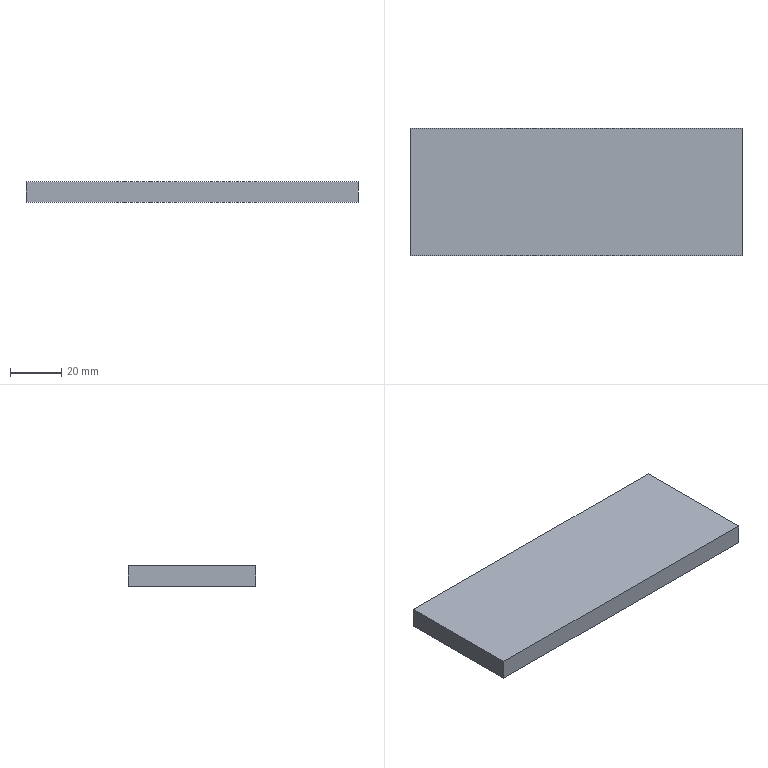Part | STEP file | 08-Steel plate 130x50x8 | 1 solid | 6 faces | box 130 x 50 x 8 mm | volume 52000 mm3 | plane 6
STEP:
#1=CARTESIAN_POINT('',(0.,0.,0.));
#2=DIRECTION('',(0.,0.,1.));
#3=DIRECTION('',(1.,0.,0.));
#4=AXIS2_PLACEMENT_3D('',#1,#2,#3);
#5=CARTESIAN_POINT('',(0.,0.,0.));
#6=VERTEX_POINT('',#5);
#7=CARTESIAN_POINT('',(0.,-50.,0.));
#8=VERTEX_POINT('',#7);
#9=CARTESIAN_POINT('',(0.,0.,0.));
#10=DIRECTION('',(0.,-1.,0.));
#11=VECTOR('',#10,1.);
#12=LINE('',#9,#11);
#13=CARTESIAN_POINT('',(0.,0.,8.));
#14=DIRECTION('',(1.,0.,0.));
#15=DIRECTION('',(0.,1.,0.));
#16=AXIS2_PLACEMENT_3D('',#13,#14,#15);
#17=PLANE('',#16);
#18=CARTESIAN_POINT('',(0.,-8.));
#19=DIRECTION('',(-1.,0.));
#20=VECTOR('',#19,1.);
#21=LINE('',#18,#20);
#22=(GEOMETRIC_REPRESENTATION_CONTEXT(2)PARAMETRIC_REPRESENTATION_CONTEXT()REPRESENTATION_CONTEXT('',''));
#23=DEFINITIONAL_REPRESENTATION('',(#21),#22);
#24=PCURVE('',#17,#23);
#25=CARTESIAN_POINT('',(0.,0.,0.));
#26=DIRECTION('',(0.,0.,1.));
#27=DIRECTION('',(1.,0.,0.));
#28=AXIS2_PLACEMENT_3D('',#25,#26,#27);
#29=PLANE('',#28);
#30=CARTESIAN_POINT('',(0.,0.));
#31=DIRECTION('',(0.,-1.));
#32=VECTOR('',#31,1.);
#33=LINE('',#30,#32);
#34=(GEOMETRIC_REPRESENTATION_CONTEXT(2)PARAMETRIC_REPRESENTATION_CONTEXT()REPRESENTATION_CONTEXT('',''));
#35=DEFINITIONAL_REPRESENTATION('',(#33),#34);
#36=PCURVE('',#29,#35);
#37=SURFACE_CURVE('',#12,(#24,#36),.PCURVE_S1.);
#38=EDGE_CURVE('',#6,#8,#37,.T.);
#39=ORIENTED_EDGE('',*,*,#38,.T.);
#40=CARTESIAN_POINT('',(0.,-50.,8.));
#41=VERTEX_POINT('',#40);
#42=CARTESIAN_POINT('',(0.,-50.,8.));
#43=DIRECTION('',(0.,0.,-1.));
#44=VECTOR('',#43,1.);
#45=LINE('',#42,#44);
#46=CARTESIAN_POINT('',(-50.,0.));
#47=DIRECTION('',(0.,-1.));
#48=VECTOR('',#47,1.);
#49=LINE('',#46,#48);
#50=(GEOMETRIC_REPRESENTATION_CONTEXT(2)PARAMETRIC_REPRESENTATION_CONTEXT()REPRESENTATION_CONTEXT('',''));
#51=DEFINITIONAL_REPRESENTATION('',(#49),#50);
#52=PCURVE('',#17,#51);
#53=CARTESIAN_POINT('',(0.,-50.,8.));
#54=DIRECTION('',(0.,1.,0.));
#55=DIRECTION('',(0.,0.,1.));
#56=AXIS2_PLACEMENT_3D('',#53,#54,#55);
#57=PLANE('',#56);
#58=CARTESIAN_POINT('',(0.,0.));
#59=DIRECTION('',(-1.,0.));
#60=VECTOR('',#59,1.);
#61=LINE('',#58,#60);
#62=(GEOMETRIC_REPRESENTATION_CONTEXT(2)PARAMETRIC_REPRESENTATION_CONTEXT()REPRESENTATION_CONTEXT('',''));
#63=DEFINITIONAL_REPRESENTATION('',(#61),#62);
#64=PCURVE('',#57,#63);
#65=SURFACE_CURVE('',#45,(#52,#64),.PCURVE_S1.);
#66=EDGE_CURVE('',#41,#8,#65,.T.);
#67=ORIENTED_EDGE('',*,*,#66,.F.);
#68=CARTESIAN_POINT('',(0.,0.,8.));
#69=VERTEX_POINT('',#68);
#70=CARTESIAN_POINT('',(0.,0.,8.));
#71=DIRECTION('',(0.,-1.,0.));
#72=VECTOR('',#71,1.);
#73=LINE('',#70,#72);
#74=CARTESIAN_POINT('',(0.,0.));
#75=DIRECTION('',(-1.,0.));
#76=VECTOR('',#75,1.);
#77=LINE('',#74,#76);
#78=(GEOMETRIC_REPRESENTATION_CONTEXT(2)PARAMETRIC_REPRESENTATION_CONTEXT()REPRESENTATION_CONTEXT('',''));
#79=DEFINITIONAL_REPRESENTATION('',(#77),#78);
#80=PCURVE('',#17,#79);
#81=CARTESIAN_POINT('',(0.,0.,8.));
#82=DIRECTION('',(0.,0.,1.));
#83=DIRECTION('',(1.,0.,0.));
#84=AXIS2_PLACEMENT_3D('',#81,#82,#83);
#85=PLANE('',#84);
#86=CARTESIAN_POINT('',(0.,0.));
#87=DIRECTION('',(0.,-1.));
#88=VECTOR('',#87,1.);
#89=LINE('',#86,#88);
#90=(GEOMETRIC_REPRESENTATION_CONTEXT(2)PARAMETRIC_REPRESENTATION_CONTEXT()REPRESENTATION_CONTEXT('',''));
#91=DEFINITIONAL_REPRESENTATION('',(#89),#90);
#92=PCURVE('',#85,#91);
#93=SURFACE_CURVE('',#73,(#80,#92),.PCURVE_S1.);
#94=EDGE_CURVE('',#69,#41,#93,.T.);
#95=ORIENTED_EDGE('',*,*,#94,.F.);
#96=CARTESIAN_POINT('',(0.,0.,8.));
#97=DIRECTION('',(0.,0.,-1.));
#98=VECTOR('',#97,1.);
#99=LINE('',#96,#98);
#100=CARTESIAN_POINT('',(0.,0.));
#101=DIRECTION('',(0.,-1.));
#102=VECTOR('',#101,1.);
#103=LINE('',#100,#102);
#104=(GEOMETRIC_REPRESENTATION_CONTEXT(2)PARAMETRIC_REPRESENTATION_CONTEXT()REPRESENTATION_CONTEXT('',''));
#105=DEFINITIONAL_REPRESENTATION('',(#103),#104);
#106=PCURVE('',#17,#105);
#107=CARTESIAN_POINT('',(0.,0.,8.));
#108=DIRECTION('',(0.,-1.,0.));
#109=DIRECTION('',(0.,0.,-1.));
#110=AXIS2_PLACEMENT_3D('',#107,#108,#109);
#111=PLANE('',#110);
#112=CARTESIAN_POINT('',(0.,0.));
#113=DIRECTION('',(1.,0.));
#114=VECTOR('',#113,1.);
#115=LINE('',#112,#114);
#116=(GEOMETRIC_REPRESENTATION_CONTEXT(2)PARAMETRIC_REPRESENTATION_CONTEXT()REPRESENTATION_CONTEXT('',''));
#117=DEFINITIONAL_REPRESENTATION('',(#115),#116);
#118=PCURVE('',#111,#117);
#119=SURFACE_CURVE('',#99,(#106,#118),.PCURVE_S1.);
#120=EDGE_CURVE('',#69,#6,#119,.T.);
#121=ORIENTED_EDGE('',*,*,#120,.T.);
#122=EDGE_LOOP('',(#39,#67,#95,#121));
#123=FACE_BOUND('',#122,.T.);
#124=ADVANCED_FACE('',(#123),#17,.F.);
#125=CARTESIAN_POINT('',(130.,-50.,0.));
#126=VERTEX_POINT('',#125);
#127=CARTESIAN_POINT('',(0.,-50.,0.));
#128=DIRECTION('',(1.,0.,0.));
#129=VECTOR('',#128,1.);
#130=LINE('',#127,#129);
#131=CARTESIAN_POINT('',(-8.,0.));
#132=DIRECTION('',(0.,1.));
#133=VECTOR('',#132,1.);
#134=LINE('',#131,#133);
#135=(GEOMETRIC_REPRESENTATION_CONTEXT(2)PARAMETRIC_REPRESENTATION_CONTEXT()REPRESENTATION_CONTEXT('',''));
#136=DEFINITIONAL_REPRESENTATION('',(#134),#135);
#137=PCURVE('',#57,#136);
#138=CARTESIAN_POINT('',(0.,-50.));
#139=DIRECTION('',(1.,0.));
#140=VECTOR('',#139,1.);
#141=LINE('',#138,#140);
#142=(GEOMETRIC_REPRESENTATION_CONTEXT(2)PARAMETRIC_REPRESENTATION_CONTEXT()REPRESENTATION_CONTEXT('',''));
#143=DEFINITIONAL_REPRESENTATION('',(#141),#142);
#144=PCURVE('',#29,#143);
#145=SURFACE_CURVE('',#130,(#137,#144),.PCURVE_S1.);
#146=EDGE_CURVE('',#8,#126,#145,.T.);
#147=ORIENTED_EDGE('',*,*,#146,.T.);
#148=CARTESIAN_POINT('',(130.,-50.,8.));
#149=VERTEX_POINT('',#148);
#150=CARTESIAN_POINT('',(130.,-50.,8.));
#151=DIRECTION('',(0.,0.,-1.));
#152=VECTOR('',#151,1.);
#153=LINE('',#150,#152);
#154=CARTESIAN_POINT('',(0.,130.));
#155=DIRECTION('',(-1.,0.));
#156=VECTOR('',#155,1.);
#157=LINE('',#154,#156);
#158=(GEOMETRIC_REPRESENTATION_CONTEXT(2)PARAMETRIC_REPRESENTATION_CONTEXT()REPRESENTATION_CONTEXT('',''));
#159=DEFINITIONAL_REPRESENTATION('',(#157),#158);
#160=PCURVE('',#57,#159);
#161=CARTESIAN_POINT('',(130.,0.,8.));
#162=DIRECTION('',(-1.,0.,0.));
#163=DIRECTION('',(0.,0.,1.));
#164=AXIS2_PLACEMENT_3D('',#161,#162,#163);
#165=PLANE('',#164);
#166=CARTESIAN_POINT('',(0.,-50.));
#167=DIRECTION('',(-1.,0.));
#168=VECTOR('',#167,1.);
#169=LINE('',#166,#168);
#170=(GEOMETRIC_REPRESENTATION_CONTEXT(2)PARAMETRIC_REPRESENTATION_CONTEXT()REPRESENTATION_CONTEXT('',''));
#171=DEFINITIONAL_REPRESENTATION('',(#169),#170);
#172=PCURVE('',#165,#171);
#173=SURFACE_CURVE('',#153,(#160,#172),.PCURVE_S1.);
#174=EDGE_CURVE('',#149,#126,#173,.T.);
#175=ORIENTED_EDGE('',*,*,#174,.F.);
#176=CARTESIAN_POINT('',(0.,-50.,8.));
#177=DIRECTION('',(1.,0.,0.));
#178=VECTOR('',#177,1.);
#179=LINE('',#176,#178);
#180=CARTESIAN_POINT('',(0.,0.));
#181=DIRECTION('',(0.,1.));
#182=VECTOR('',#181,1.);
#183=LINE('',#180,#182);
#184=(GEOMETRIC_REPRESENTATION_CONTEXT(2)PARAMETRIC_REPRESENTATION_CONTEXT()REPRESENTATION_CONTEXT('',''));
#185=DEFINITIONAL_REPRESENTATION('',(#183),#184);
#186=PCURVE('',#57,#185);
#187=CARTESIAN_POINT('',(0.,-50.));
#188=DIRECTION('',(1.,0.));
#189=VECTOR('',#188,1.);
#190=LINE('',#187,#189);
#191=(GEOMETRIC_REPRESENTATION_CONTEXT(2)PARAMETRIC_REPRESENTATION_CONTEXT()REPRESENTATION_CONTEXT('',''));
#192=DEFINITIONAL_REPRESENTATION('',(#190),#191);
#193=PCURVE('',#85,#192);
#194=SURFACE_CURVE('',#179,(#186,#193),.PCURVE_S1.);
#195=EDGE_CURVE('',#41,#149,#194,.T.);
#196=ORIENTED_EDGE('',*,*,#195,.F.);
#197=ORIENTED_EDGE('',*,*,#66,.T.);
#198=EDGE_LOOP('',(#147,#175,#196,#197));
#199=FACE_BOUND('',#198,.T.);
#200=ADVANCED_FACE('',(#199),#57,.F.);
#201=CARTESIAN_POINT('',(130.,0.,0.));
#202=VERTEX_POINT('',#201);
#203=CARTESIAN_POINT('',(130.,0.,0.));
#204=DIRECTION('',(0.,1.,0.));
#205=VECTOR('',#204,1.);
#206=LINE('',#203,#205);
#207=CARTESIAN_POINT('',(-8.,0.));
#208=DIRECTION('',(0.,1.));
#209=VECTOR('',#208,1.);
#210=LINE('',#207,#209);
#211=(GEOMETRIC_REPRESENTATION_CONTEXT(2)PARAMETRIC_REPRESENTATION_CONTEXT()REPRESENTATION_CONTEXT('',''));
#212=DEFINITIONAL_REPRESENTATION('',(#210),#211);
#213=PCURVE('',#165,#212);
#214=CARTESIAN_POINT('',(130.,0.));
#215=DIRECTION('',(0.,1.));
#216=VECTOR('',#215,1.);
#217=LINE('',#214,#216);
#218=(GEOMETRIC_REPRESENTATION_CONTEXT(2)PARAMETRIC_REPRESENTATION_CONTEXT()REPRESENTATION_CONTEXT('',''));
#219=DEFINITIONAL_REPRESENTATION('',(#217),#218);
#220=PCURVE('',#29,#219);
#221=SURFACE_CURVE('',#206,(#213,#220),.PCURVE_S1.);
#222=EDGE_CURVE('',#126,#202,#221,.T.);
#223=ORIENTED_EDGE('',*,*,#222,.T.);
#224=CARTESIAN_POINT('',(130.,0.,8.));
#225=VERTEX_POINT('',#224);
#226=CARTESIAN_POINT('',(130.,0.,8.));
#227=DIRECTION('',(0.,0.,-1.));
#228=VECTOR('',#227,1.);
#229=LINE('',#226,#228);
#230=CARTESIAN_POINT('',(0.,0.));
#231=DIRECTION('',(-1.,0.));
#232=VECTOR('',#231,1.);
#233=LINE('',#230,#232);
#234=(GEOMETRIC_REPRESENTATION_CONTEXT(2)PARAMETRIC_REPRESENTATION_CONTEXT()REPRESENTATION_CONTEXT('',''));
#235=DEFINITIONAL_REPRESENTATION('',(#233),#234);
#236=PCURVE('',#165,#235);
#237=CARTESIAN_POINT('',(0.,130.));
#238=DIRECTION('',(1.,0.));
#239=VECTOR('',#238,1.);
#240=LINE('',#237,#239);
#241=(GEOMETRIC_REPRESENTATION_CONTEXT(2)PARAMETRIC_REPRESENTATION_CONTEXT()REPRESENTATION_CONTEXT('',''));
#242=DEFINITIONAL_REPRESENTATION('',(#240),#241);
#243=PCURVE('',#111,#242);
#244=SURFACE_CURVE('',#229,(#236,#243),.PCURVE_S1.);
#245=EDGE_CURVE('',#225,#202,#244,.T.);
#246=ORIENTED_EDGE('',*,*,#245,.F.);
#247=CARTESIAN_POINT('',(130.,0.,8.));
#248=DIRECTION('',(0.,1.,0.));
#249=VECTOR('',#248,1.);
#250=LINE('',#247,#249);
#251=CARTESIAN_POINT('',(0.,0.));
#252=DIRECTION('',(0.,1.));
#253=VECTOR('',#252,1.);
#254=LINE('',#251,#253);
#255=(GEOMETRIC_REPRESENTATION_CONTEXT(2)PARAMETRIC_REPRESENTATION_CONTEXT()REPRESENTATION_CONTEXT('',''));
#256=DEFINITIONAL_REPRESENTATION('',(#254),#255);
#257=PCURVE('',#165,#256);
#258=CARTESIAN_POINT('',(130.,0.));
#259=DIRECTION('',(0.,1.));
#260=VECTOR('',#259,1.);
#261=LINE('',#258,#260);
#262=(GEOMETRIC_REPRESENTATION_CONTEXT(2)PARAMETRIC_REPRESENTATION_CONTEXT()REPRESENTATION_CONTEXT('',''));
#263=DEFINITIONAL_REPRESENTATION('',(#261),#262);
#264=PCURVE('',#85,#263);
#265=SURFACE_CURVE('',#250,(#257,#264),.PCURVE_S1.);
#266=EDGE_CURVE('',#149,#225,#265,.T.);
#267=ORIENTED_EDGE('',*,*,#266,.F.);
#268=ORIENTED_EDGE('',*,*,#174,.T.);
#269=EDGE_LOOP('',(#223,#246,#267,#268));
#270=FACE_BOUND('',#269,.T.);
#271=ADVANCED_FACE('',(#270),#165,.F.);
#272=CARTESIAN_POINT('',(0.,0.,0.));
#273=DIRECTION('',(-1.,0.,0.));
#274=VECTOR('',#273,1.);
#275=LINE('',#272,#274);
#276=CARTESIAN_POINT('',(8.,0.));
#277=DIRECTION('',(0.,-1.));
#278=VECTOR('',#277,1.);
#279=LINE('',#276,#278);
#280=(GEOMETRIC_REPRESENTATION_CONTEXT(2)PARAMETRIC_REPRESENTATION_CONTEXT()REPRESENTATION_CONTEXT('',''));
#281=DEFINITIONAL_REPRESENTATION('',(#279),#280);
#282=PCURVE('',#111,#281);
#283=CARTESIAN_POINT('',(0.,0.));
#284=DIRECTION('',(-1.,0.));
#285=VECTOR('',#284,1.);
#286=LINE('',#283,#285);
#287=(GEOMETRIC_REPRESENTATION_CONTEXT(2)PARAMETRIC_REPRESENTATION_CONTEXT()REPRESENTATION_CONTEXT('',''));
#288=DEFINITIONAL_REPRESENTATION('',(#286),#287);
#289=PCURVE('',#29,#288);
#290=SURFACE_CURVE('',#275,(#282,#289),.PCURVE_S1.);
#291=EDGE_CURVE('',#202,#6,#290,.T.);
#292=ORIENTED_EDGE('',*,*,#291,.T.);
#293=ORIENTED_EDGE('',*,*,#120,.F.);
#294=CARTESIAN_POINT('',(0.,0.,8.));
#295=DIRECTION('',(-1.,0.,0.));
#296=VECTOR('',#295,1.);
#297=LINE('',#294,#296);
#298=CARTESIAN_POINT('',(0.,0.));
#299=DIRECTION('',(0.,-1.));
#300=VECTOR('',#299,1.);
#301=LINE('',#298,#300);
#302=(GEOMETRIC_REPRESENTATION_CONTEXT(2)PARAMETRIC_REPRESENTATION_CONTEXT()REPRESENTATION_CONTEXT('',''));
#303=DEFINITIONAL_REPRESENTATION('',(#301),#302);
#304=PCURVE('',#111,#303);
#305=CARTESIAN_POINT('',(0.,0.));
#306=DIRECTION('',(-1.,0.));
#307=VECTOR('',#306,1.);
#308=LINE('',#305,#307);
#309=(GEOMETRIC_REPRESENTATION_CONTEXT(2)PARAMETRIC_REPRESENTATION_CONTEXT()REPRESENTATION_CONTEXT('',''));
#310=DEFINITIONAL_REPRESENTATION('',(#308),#309);
#311=PCURVE('',#85,#310);
#312=SURFACE_CURVE('',#297,(#304,#311),.PCURVE_S1.);
#313=EDGE_CURVE('',#225,#69,#312,.T.);
#314=ORIENTED_EDGE('',*,*,#313,.F.);
#315=ORIENTED_EDGE('',*,*,#245,.T.);
#316=EDGE_LOOP('',(#292,#293,#314,#315));
#317=FACE_BOUND('',#316,.T.);
#318=ADVANCED_FACE('',(#317),#111,.F.);
#319=ORIENTED_EDGE('',*,*,#94,.T.);
#320=ORIENTED_EDGE('',*,*,#195,.T.);
#321=ORIENTED_EDGE('',*,*,#266,.T.);
#322=ORIENTED_EDGE('',*,*,#313,.T.);
#323=EDGE_LOOP('',(#319,#320,#321,#322));
#324=FACE_BOUND('',#323,.T.);
#325=ADVANCED_FACE('',(#324),#85,.T.);
#326=ORIENTED_EDGE('',*,*,#38,.F.);
#327=ORIENTED_EDGE('',*,*,#291,.F.);
#328=ORIENTED_EDGE('',*,*,#222,.F.);
#329=ORIENTED_EDGE('',*,*,#146,.F.);
#330=EDGE_LOOP('',(#326,#327,#328,#329));
#331=FACE_BOUND('',#330,.T.);
#332=ADVANCED_FACE('',(#331),#29,.F.);
#333=CLOSED_SHELL('',(#124,#200,#271,#318,#325,#332));
#334=MANIFOLD_SOLID_BREP('',#333);
#335=(LENGTH_UNIT()NAMED_UNIT(*)SI_UNIT(.MILLI.,.METRE.));
#336=UNCERTAINTY_MEASURE_WITH_UNIT(LENGTH_MEASURE(0.0000001),#335,'','');
#337=(NAMED_UNIT(*)PLANE_ANGLE_UNIT()SI_UNIT($,.RADIAN.));
#338=(NAMED_UNIT(*)SI_UNIT($,.STERADIAN.)SOLID_ANGLE_UNIT());
#339=(GEOMETRIC_REPRESENTATION_CONTEXT(3)GLOBAL_UNCERTAINTY_ASSIGNED_CONTEXT((#336))GLOBAL_UNIT_ASSIGNED_CONTEXT((#335,#337,#338))REPRESENTATION_CONTEXT('',''));
#340=ADVANCED_BREP_SHAPE_REPRESENTATION('',(#4,#334),#339);